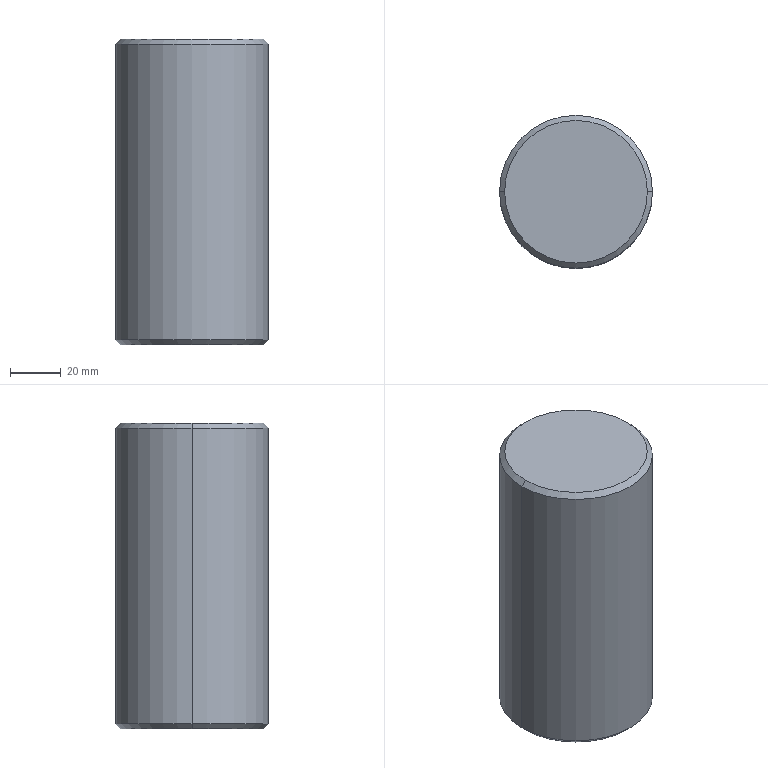Part | STEP file | 4-20.sldasm-Part-324 | 1 solid | 8 faces | box 60 x 60 x 120 mm | volume 338555 mm3 | cone 4 | cylinder 2 | plane 2 | commonest cylinder face diameters 60 x2
STEP:
#1=CARTESIAN_POINT('',(23.,275.,-20.));
#2=VERTEX_POINT('',#1);
#3=CARTESIAN_POINT('',(-33.,275.,-20.));
#4=VERTEX_POINT('',#3);
#5=CARTESIAN_POINT('',(-5.,275.,-20.));
#6=DIRECTION('',(0.,0.,1.));
#7=DIRECTION('',(1.,0.,0.));
#8=AXIS2_PLACEMENT_3D('',#5,#6,#7);
#9=CIRCLE('',#8,28.);
#10=EDGE_CURVE('',#2,#4,#9,.T.);
#11=ORIENTED_EDGE('',*,*,#10,.F.);
#12=CARTESIAN_POINT('',(25.,275.,-22.));
#13=VERTEX_POINT('',#12);
#14=CARTESIAN_POINT('',(23.,275.,-20.));
#15=DIRECTION('',(0.7071,0.,-0.7071));
#16=VECTOR('',#15,1000.);
#17=LINE('',#14,#16);
#18=EDGE_CURVE('',#2,#13,#17,.T.);
#19=ORIENTED_EDGE('',*,*,#18,.T.);
#20=CARTESIAN_POINT('',(-35.,275.,-22.));
#21=VERTEX_POINT('',#20);
#22=CARTESIAN_POINT('',(-5.,275.,-22.));
#23=DIRECTION('',(0.,0.,-1.));
#24=DIRECTION('',(1.,0.,0.));
#25=AXIS2_PLACEMENT_3D('',#22,#23,#24);
#26=CIRCLE('',#25,30.);
#27=EDGE_CURVE('',#21,#13,#26,.T.);
#28=ORIENTED_EDGE('',*,*,#27,.F.);
#29=CARTESIAN_POINT('',(-33.,275.,-20.));
#30=DIRECTION('',(-0.7071,0.,-0.7071));
#31=VECTOR('',#30,1000.);
#32=LINE('',#29,#31);
#33=EDGE_CURVE('',#4,#21,#32,.T.);
#34=ORIENTED_EDGE('',*,*,#33,.F.);
#35=EDGE_LOOP('',(#11,#19,#28,#34));
#36=FACE_OUTER_BOUND('',#35,.T.);
#37=CARTESIAN_POINT('',(-5.,275.,-20.));
#38=DIRECTION('',(0.,0.,-1.));
#39=DIRECTION('',(-1.,0.,0.));
#40=AXIS2_PLACEMENT_3D('',#37,#38,#39);
#41=CONICAL_SURFACE('',#40,28.,0.7854);
#42=ADVANCED_FACE('',(#36),#41,.T.);
#43=CARTESIAN_POINT('',(-33.,275.,-140.));
#44=VERTEX_POINT('',#43);
#45=CARTESIAN_POINT('',(23.,275.,-140.));
#46=VERTEX_POINT('',#45);
#47=CARTESIAN_POINT('',(-5.,275.,-140.));
#48=DIRECTION('',(0.,0.,-1.));
#49=DIRECTION('',(1.,0.,0.));
#50=AXIS2_PLACEMENT_3D('',#47,#48,#49);
#51=CIRCLE('',#50,28.);
#52=EDGE_CURVE('',#44,#46,#51,.T.);
#53=ORIENTED_EDGE('',*,*,#52,.F.);
#54=CARTESIAN_POINT('',(-35.,275.,-138.));
#55=VERTEX_POINT('',#54);
#56=CARTESIAN_POINT('',(-33.,275.,-140.));
#57=DIRECTION('',(-0.7071,0.,0.7071));
#58=VECTOR('',#57,1000.);
#59=LINE('',#56,#58);
#60=EDGE_CURVE('',#44,#55,#59,.T.);
#61=ORIENTED_EDGE('',*,*,#60,.T.);
#62=CARTESIAN_POINT('',(25.,275.,-138.));
#63=VERTEX_POINT('',#62);
#64=CARTESIAN_POINT('',(-5.,275.,-138.));
#65=DIRECTION('',(0.,0.,1.));
#66=DIRECTION('',(1.,0.,0.));
#67=AXIS2_PLACEMENT_3D('',#64,#65,#66);
#68=CIRCLE('',#67,30.);
#69=EDGE_CURVE('',#63,#55,#68,.T.);
#70=ORIENTED_EDGE('',*,*,#69,.F.);
#71=CARTESIAN_POINT('',(23.,275.,-140.));
#72=DIRECTION('',(0.7071,0.,0.7071));
#73=VECTOR('',#72,1000.);
#74=LINE('',#71,#73);
#75=EDGE_CURVE('',#46,#63,#74,.T.);
#76=ORIENTED_EDGE('',*,*,#75,.F.);
#77=EDGE_LOOP('',(#53,#61,#70,#76));
#78=FACE_OUTER_BOUND('',#77,.T.);
#79=CARTESIAN_POINT('',(-5.,275.,-140.));
#80=DIRECTION('',(0.,0.,1.));
#81=DIRECTION('',(1.,0.,0.));
#82=AXIS2_PLACEMENT_3D('',#79,#80,#81);
#83=CONICAL_SURFACE('',#82,28.,0.7854);
#84=ADVANCED_FACE('',(#78),#83,.T.);
#85=ORIENTED_EDGE('',*,*,#69,.T.);
#86=CARTESIAN_POINT('',(-35.,275.,-679.868));
#87=DIRECTION('',(0.,0.,1.));
#88=VECTOR('',#87,1000.);
#89=LINE('',#86,#88);
#90=EDGE_CURVE('',#55,#21,#89,.T.);
#91=ORIENTED_EDGE('',*,*,#90,.T.);
#92=ORIENTED_EDGE('',*,*,#27,.T.);
#93=CARTESIAN_POINT('',(25.,275.,-679.868));
#94=DIRECTION('',(0.,0.,1.));
#95=VECTOR('',#94,1000.);
#96=LINE('',#93,#95);
#97=EDGE_CURVE('',#63,#13,#96,.T.);
#98=ORIENTED_EDGE('',*,*,#97,.F.);
#99=EDGE_LOOP('',(#85,#91,#92,#98));
#100=FACE_OUTER_BOUND('',#99,.T.);
#101=CARTESIAN_POINT('',(-5.,275.,-679.868));
#102=DIRECTION('',(0.,0.,1.));
#103=DIRECTION('',(1.,0.,0.));
#104=AXIS2_PLACEMENT_3D('',#101,#102,#103);
#105=CYLINDRICAL_SURFACE('',#104,30.);
#106=ADVANCED_FACE('',(#100),#105,.T.);
#107=CARTESIAN_POINT('',(-5.,275.,-140.));
#108=DIRECTION('',(0.,0.,-1.));
#109=DIRECTION('',(1.,0.,0.));
#110=AXIS2_PLACEMENT_3D('',#107,#108,#109);
#111=CIRCLE('',#110,28.);
#112=EDGE_CURVE('',#46,#44,#111,.T.);
#113=ORIENTED_EDGE('',*,*,#112,.T.);
#114=ORIENTED_EDGE('',*,*,#52,.T.);
#115=EDGE_LOOP('',(#113,#114));
#116=FACE_OUTER_BOUND('',#115,.T.);
#117=CARTESIAN_POINT('',(-421.067,-693.4,-140.));
#118=DIRECTION('',(0.,0.,1.));
#119=DIRECTION('',(0.,-1.,0.));
#120=AXIS2_PLACEMENT_3D('',#117,#118,#119);
#121=PLANE('',#120);
#122=ADVANCED_FACE('',(#116),#121,.F.);
#123=CARTESIAN_POINT('',(-5.,275.,-20.));
#124=DIRECTION('',(0.,0.,1.));
#125=DIRECTION('',(1.,0.,0.));
#126=AXIS2_PLACEMENT_3D('',#123,#124,#125);
#127=CIRCLE('',#126,28.);
#128=EDGE_CURVE('',#4,#2,#127,.T.);
#129=ORIENTED_EDGE('',*,*,#128,.T.);
#130=ORIENTED_EDGE('',*,*,#10,.T.);
#131=EDGE_LOOP('',(#129,#130));
#132=FACE_OUTER_BOUND('',#131,.T.);
#133=CARTESIAN_POINT('',(-5.,275.,-20.));
#134=DIRECTION('',(0.,0.,1.));
#135=DIRECTION('',(1.,0.,0.));
#136=AXIS2_PLACEMENT_3D('',#133,#134,#135);
#137=PLANE('',#136);
#138=ADVANCED_FACE('',(#132),#137,.T.);
#139=ORIENTED_EDGE('',*,*,#90,.F.);
#140=CARTESIAN_POINT('',(-5.,275.,-138.));
#141=DIRECTION('',(0.,0.,1.));
#142=DIRECTION('',(1.,0.,0.));
#143=AXIS2_PLACEMENT_3D('',#140,#141,#142);
#144=CIRCLE('',#143,30.);
#145=EDGE_CURVE('',#55,#63,#144,.T.);
#146=ORIENTED_EDGE('',*,*,#145,.T.);
#147=ORIENTED_EDGE('',*,*,#97,.T.);
#148=CARTESIAN_POINT('',(-5.,275.,-22.));
#149=DIRECTION('',(0.,0.,-1.));
#150=DIRECTION('',(1.,0.,0.));
#151=AXIS2_PLACEMENT_3D('',#148,#149,#150);
#152=CIRCLE('',#151,30.);
#153=EDGE_CURVE('',#13,#21,#152,.T.);
#154=ORIENTED_EDGE('',*,*,#153,.T.);
#155=EDGE_LOOP('',(#139,#146,#147,#154));
#156=FACE_OUTER_BOUND('',#155,.T.);
#157=CARTESIAN_POINT('',(-5.,275.,-679.868));
#158=DIRECTION('',(0.,0.,1.));
#159=DIRECTION('',(1.,0.,0.));
#160=AXIS2_PLACEMENT_3D('',#157,#158,#159);
#161=CYLINDRICAL_SURFACE('',#160,30.);
#162=ADVANCED_FACE('',(#156),#161,.T.);
#163=ORIENTED_EDGE('',*,*,#60,.F.);
#164=ORIENTED_EDGE('',*,*,#112,.F.);
#165=ORIENTED_EDGE('',*,*,#75,.T.);
#166=ORIENTED_EDGE('',*,*,#145,.F.);
#167=EDGE_LOOP('',(#163,#164,#165,#166));
#168=FACE_OUTER_BOUND('',#167,.T.);
#169=CARTESIAN_POINT('',(-5.,275.,-140.));
#170=DIRECTION('',(0.,0.,1.));
#171=DIRECTION('',(1.,0.,0.));
#172=AXIS2_PLACEMENT_3D('',#169,#170,#171);
#173=CONICAL_SURFACE('',#172,28.,0.7854);
#174=ADVANCED_FACE('',(#168),#173,.T.);
#175=ORIENTED_EDGE('',*,*,#18,.F.);
#176=ORIENTED_EDGE('',*,*,#128,.F.);
#177=ORIENTED_EDGE('',*,*,#33,.T.);
#178=ORIENTED_EDGE('',*,*,#153,.F.);
#179=EDGE_LOOP('',(#175,#176,#177,#178));
#180=FACE_OUTER_BOUND('',#179,.T.);
#181=CARTESIAN_POINT('',(-5.,275.,-20.));
#182=DIRECTION('',(0.,0.,-1.));
#183=DIRECTION('',(-1.,0.,0.));
#184=AXIS2_PLACEMENT_3D('',#181,#182,#183);
#185=CONICAL_SURFACE('',#184,28.,0.7854);
#186=ADVANCED_FACE('',(#180),#185,.T.);
#187=CLOSED_SHELL('',(#42,#84,#106,#122,#138,#162,#174,#186));
#188=MANIFOLD_SOLID_BREP('',#187);
#189=CARTESIAN_POINT('',(0.,0.,0.));
#190=DIRECTION('',(0.,0.,1.));
#191=DIRECTION('',(1.,0.,0.));
#192=AXIS2_PLACEMENT_3D('',#189,#190,#191);
#193=(LENGTH_UNIT()NAMED_UNIT(*)SI_UNIT(.MILLI.,.METRE.));
#194=UNCERTAINTY_MEASURE_WITH_UNIT(LENGTH_MEASURE(0.00001),#193,'','');
#195=(NAMED_UNIT(*)PLANE_ANGLE_UNIT()SI_UNIT($,.RADIAN.));
#196=(NAMED_UNIT(*)SI_UNIT($,.STERADIAN.)SOLID_ANGLE_UNIT());
#197=(GEOMETRIC_REPRESENTATION_CONTEXT(3)GLOBAL_UNCERTAINTY_ASSIGNED_CONTEXT((#194))GLOBAL_UNIT_ASSIGNED_CONTEXT((#193,#195,#196))REPRESENTATION_CONTEXT('',''));
#198=ADVANCED_BREP_SHAPE_REPRESENTATION('',(#188,#192),#197);